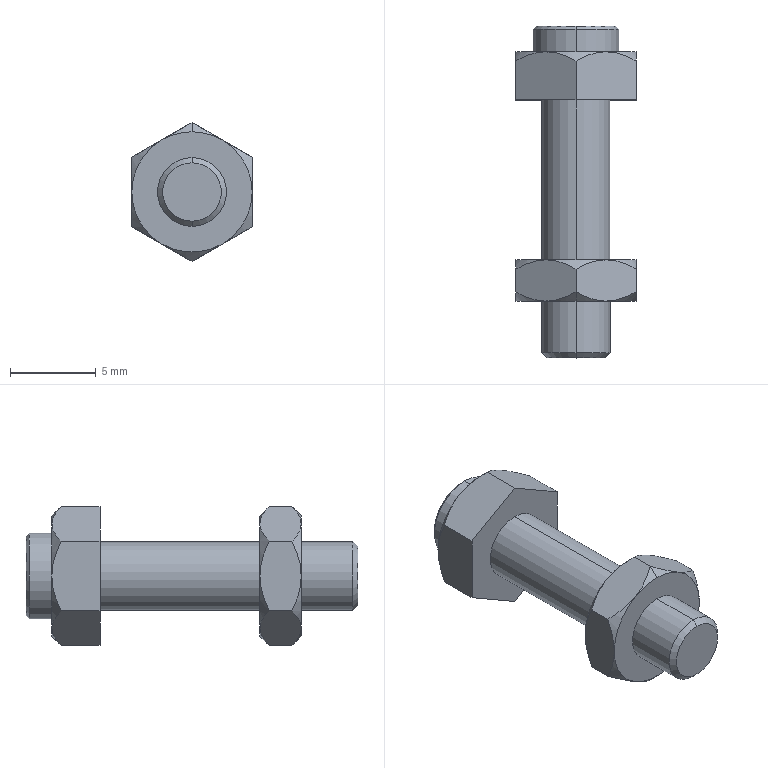Part | STEP file | Shoulder stop bolt M4×20 | 1 solid | 49 faces | box 7 x 19.3 x 8.083 mm | volume 405.674 mm3 | cone 25 | plane 18 | cylinder 6 | commonest cylinder face diameters 4 x4 5 x2